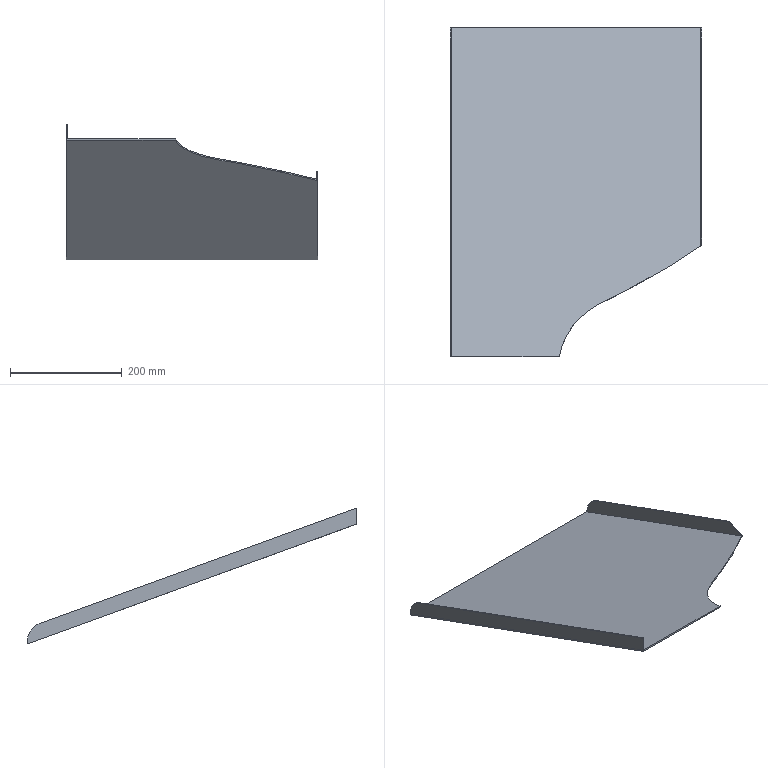Part | NX | features solid 2 | 1 solid | 15 faces | box 450 x 590 x 243.475 mm | volume 550261 mm3 | plane 11 | spline 2 | cylinder 2 | commonest cylinder face diameters 70 x2
STEP:
#1=CARTESIAN_POINT('',(-1002.,620.,-276.254));
#2=VERTEX_POINT('',#1);
#3=CARTESIAN_POINT('',(-1448.,620.,-276.254));
#4=VERTEX_POINT('',#3);
#5=CARTESIAN_POINT('',(-1000.,620.,-276.254));
#6=DIRECTION('',(-1.,0.,0.));
#7=VECTOR('',#6,1000.);
#8=LINE('',#5,#7);
#9=EDGE_CURVE('',#2,#4,#8,.T.);
#10=ORIENTED_EDGE('',*,*,#9,.T.);
#11=CARTESIAN_POINT('',(-1448.,30.,-61.511));
#12=VERTEX_POINT('',#11);
#13=CARTESIAN_POINT('',(-1448.,10.,-54.232));
#14=DIRECTION('',(0.,0.9397,-0.342));
#15=VECTOR('',#14,1000.);
#16=LINE('',#13,#15);
#17=EDGE_CURVE('',#12,#4,#16,.T.);
#18=ORIENTED_EDGE('',*,*,#17,.F.);
#19=CARTESIAN_POINT('',(-1254.916,30.,-61.511));
#20=VERTEX_POINT('',#19);
#21=CARTESIAN_POINT('',(-1445.,30.,-61.511));
#22=DIRECTION('',(1.,0.,0.));
#23=VECTOR('',#22,1000.);
#24=LINE('',#21,#23);
#25=EDGE_CURVE('',#20,#12,#24,.F.);
#26=ORIENTED_EDGE('',*,*,#25,.F.);
#27=CARTESIAN_POINT('',(-1059.954,190.696,-120.));
#28=VERTEX_POINT('',#27);
#29=CARTESIAN_POINT('',(-1059.954,190.696,-120.));
#30=CARTESIAN_POINT('',(-1064.698,187.84,-118.96));
#31=CARTESIAN_POINT('',(-1074.259,182.234,-116.92));
#32=CARTESIAN_POINT('',(-1088.653,173.903,-113.888));
#33=CARTESIAN_POINT('',(-1103.077,165.617,-110.872));
#34=CARTESIAN_POINT('',(-1122.557,154.937,-106.985));
#35=CARTESIAN_POINT('',(-1147.26,142.109,-102.316));
#36=CARTESIAN_POINT('',(-1172.64,130.297,-98.016));
#37=CARTESIAN_POINT('',(-1192.179,119.686,-94.154));
#38=CARTESIAN_POINT('',(-1205.944,110.685,-90.878));
#39=CARTESIAN_POINT('',(-1218.377,100.126,-87.035));
#40=CARTESIAN_POINT('',(-1229.411,87.869,-82.574));
#41=CARTESIAN_POINT('',(-1238.508,74.677,-77.773));
#42=CARTESIAN_POINT('',(-1244.626,62.872,-73.476));
#43=CARTESIAN_POINT('',(-1248.718,52.937,-69.86));
#44=CARTESIAN_POINT('',(-1252.053,42.833,-66.182));
#45=CARTESIAN_POINT('',(-1253.907,35.157,-63.388));
#46=CARTESIAN_POINT('',(-1254.916,30.,-61.511));
#47=B_SPLINE_CURVE_WITH_KNOTS('',3,(#29,#30,#31,#32,#33,#34,#35,#36,#37,#38,#39,#40,#41,#42,#43,#44,#45,#46),.UNSPECIFIED.,.F.,.F.,(4,1,1,1,1,1,1,1,1,1,1,1,1,1,1,4),(1.07,1.086,1.103,1.12,1.137,1.171,1.205,1.222,1.239,1.256,1.273,1.289,1.306,1.315,1.323,1.34),.UNSPECIFIED.);
#48=EDGE_CURVE('',#20,#28,#47,.F.);
#49=ORIENTED_EDGE('',*,*,#48,.T.);
#50=CARTESIAN_POINT('',(-1000.,229.424,-134.096));
#51=VERTEX_POINT('',#50);
#52=CARTESIAN_POINT('',(-1000.,229.424,-134.096));
#53=CARTESIAN_POINT('',(-1009.962,222.922,-131.729));
#54=CARTESIAN_POINT('',(-1029.91,209.956,-127.01));
#55=CARTESIAN_POINT('',(-1049.758,196.836,-122.235));
#56=CARTESIAN_POINT('',(-1059.954,190.696,-120.));
#57=B_SPLINE_CURVE_WITH_KNOTS('',3,(#52,#53,#54,#55,#56),.UNSPECIFIED.,.F.,.F.,(4,1,4),(0.3322,0.3686,0.405),.UNSPECIFIED.);
#58=EDGE_CURVE('',#51,#28,#57,.T.);
#59=ORIENTED_EDGE('',*,*,#58,.F.);
#60=CARTESIAN_POINT('',(-1002.,229.424,-134.096));
#61=VERTEX_POINT('',#60);
#62=CARTESIAN_POINT('',(-1000.,229.424,-134.096));
#63=DIRECTION('',(1.,0.,0.));
#64=VECTOR('',#63,1000.);
#65=LINE('',#62,#64);
#66=EDGE_CURVE('',#51,#61,#65,.F.);
#67=ORIENTED_EDGE('',*,*,#66,.T.);
#68=CARTESIAN_POINT('',(-1002.,229.424,-134.096));
#69=DIRECTION('',(0.,0.9397,-0.342));
#70=VECTOR('',#69,1000.);
#71=LINE('',#68,#70);
#72=EDGE_CURVE('',#61,#2,#71,.T.);
#73=ORIENTED_EDGE('',*,*,#72,.T.);
#74=EDGE_LOOP('',(#10,#18,#26,#49,#59,#67,#73));
#75=FACE_BOUND('',#74,.T.);
#76=CARTESIAN_POINT('',(-1000.,352.962,-179.06));
#77=DIRECTION('',(0.,-0.342,-0.9397));
#78=DIRECTION('',(0.,0.9397,-0.342));
#79=AXIS2_PLACEMENT_3D('',#76,#77,#78);
#80=PLANE('',#79);
#81=ADVANCED_FACE('',(#75),#80,.F.);
#82=CARTESIAN_POINT('',(-1069.813,184.849,-120.));
#83=VERTEX_POINT('',#82);
#84=CARTESIAN_POINT('',(-1000.,229.424,-136.224));
#85=VERTEX_POINT('',#84);
#86=CARTESIAN_POINT('',(-1069.813,184.849,-120.));
#87=CARTESIAN_POINT('',(-1063.841,188.35,-121.274));
#88=CARTESIAN_POINT('',(-1051.942,195.415,-123.846));
#89=CARTESIAN_POINT('',(-1028.916,210.612,-129.377));
#90=CARTESIAN_POINT('',(-1011.554,221.882,-133.479));
#91=CARTESIAN_POINT('',(-1000.,229.424,-136.224));
#92=B_SPLINE_CURVE_WITH_KNOTS('',3,(#86,#87,#88,#89,#90,#91),.UNSPECIFIED.,.F.,.F.,(4,1,1,4),(0.,0.0211,0.0422,0.0844),.UNSPECIFIED.);
#93=EDGE_CURVE('',#83,#85,#92,.T.);
#94=ORIENTED_EDGE('',*,*,#93,.F.);
#95=CARTESIAN_POINT('',(-1254.916,30.,-63.64));
#96=VERTEX_POINT('',#95);
#97=CARTESIAN_POINT('',(-1069.813,184.849,-120.));
#98=CARTESIAN_POINT('',(-1074.377,182.173,-119.026));
#99=CARTESIAN_POINT('',(-1083.541,176.877,-117.099));
#100=CARTESIAN_POINT('',(-1101.846,166.25,-113.231));
#101=CARTESIAN_POINT('',(-1125.083,153.491,-108.587));
#102=CARTESIAN_POINT('',(-1153.595,139.117,-103.355));
#103=CARTESIAN_POINT('',(-1177.787,127.749,-99.218));
#104=CARTESIAN_POINT('',(-1196.15,117.253,-95.397));
#105=CARTESIAN_POINT('',(-1209.224,108.178,-92.094));
#106=CARTESIAN_POINT('',(-1220.824,97.576,-88.235));
#107=CARTESIAN_POINT('',(-1230.91,85.914,-83.991));
#108=CARTESIAN_POINT('',(-1239.501,72.925,-79.263));
#109=CARTESIAN_POINT('',(-1246.413,59.227,-74.278));
#110=CARTESIAN_POINT('',(-1251.568,44.932,-69.074));
#111=CARTESIAN_POINT('',(-1253.944,34.97,-65.449));
#112=CARTESIAN_POINT('',(-1254.916,30.,-63.64));
#113=B_SPLINE_CURVE_WITH_KNOTS('',3,(#97,#98,#99,#100,#101,#102,#103,#104,#105,#106,#107,#108,#109,#110,#111,#112),.UNSPECIFIED.,.F.,.F.,(4,1,1,1,1,1,1,1,1,1,1,1,1,4),(1.112,1.128,1.144,1.177,1.209,1.241,1.257,1.274,1.29,1.306,1.322,1.338,1.354,1.371),.UNSPECIFIED.);
#114=EDGE_CURVE('',#83,#96,#113,.T.);
#115=ORIENTED_EDGE('',*,*,#114,.T.);
#116=CARTESIAN_POINT('',(-1450.,30.,-63.64));
#117=VERTEX_POINT('',#116);
#118=CARTESIAN_POINT('',(-1000.,30.,-63.64));
#119=DIRECTION('',(-1.,0.,0.));
#120=VECTOR('',#119,1000.);
#121=LINE('',#118,#120);
#122=EDGE_CURVE('',#96,#117,#121,.T.);
#123=ORIENTED_EDGE('',*,*,#122,.T.);
#124=CARTESIAN_POINT('',(-1450.,620.,-278.382));
#125=VERTEX_POINT('',#124);
#126=CARTESIAN_POINT('',(-1450.,352.278,-180.939));
#127=DIRECTION('',(0.,-0.9397,0.342));
#128=VECTOR('',#127,1000.);
#129=LINE('',#126,#128);
#130=EDGE_CURVE('',#117,#125,#129,.F.);
#131=ORIENTED_EDGE('',*,*,#130,.T.);
#132=CARTESIAN_POINT('',(-1000.,620.,-278.382));
#133=VERTEX_POINT('',#132);
#134=CARTESIAN_POINT('',(50.,620.,-278.382));
#135=DIRECTION('',(1.,0.,0.));
#136=VECTOR('',#135,1000.);
#137=LINE('',#134,#136);
#138=EDGE_CURVE('',#133,#125,#137,.F.);
#139=ORIENTED_EDGE('',*,*,#138,.F.);
#140=CARTESIAN_POINT('',(-1000.,352.278,-180.939));
#141=DIRECTION('',(0.,0.9397,-0.342));
#142=VECTOR('',#141,1000.);
#143=LINE('',#140,#142);
#144=EDGE_CURVE('',#85,#133,#143,.T.);
#145=ORIENTED_EDGE('',*,*,#144,.F.);
#146=EDGE_LOOP('',(#94,#115,#123,#131,#139,#145));
#147=FACE_BOUND('',#146,.T.);
#148=CARTESIAN_POINT('',(-1000.,352.278,-180.939));
#149=DIRECTION('',(0.,-0.342,-0.9397));
#150=DIRECTION('',(0.,0.9397,-0.342));
#151=AXIS2_PLACEMENT_3D('',#148,#149,#150);
#152=PLANE('',#151);
#153=ADVANCED_FACE('',(#147),#152,.T.);
#154=CARTESIAN_POINT('',(-1000.,261.467,-119.154));
#155=VERTEX_POINT('',#154);
#156=CARTESIAN_POINT('',(-1000.,596.971,-241.267));
#157=VERTEX_POINT('',#156);
#158=CARTESIAN_POINT('',(-1000.,237.975,-110.603));
#159=DIRECTION('',(0.,0.9397,-0.342));
#160=VECTOR('',#159,1000.);
#161=LINE('',#158,#160);
#162=EDGE_CURVE('',#155,#157,#161,.T.);
#163=ORIENTED_EDGE('',*,*,#162,.F.);
#164=CARTESIAN_POINT('',(-1000.,312.393,-95.407));
#165=DIRECTION('',(0.,0.9063,0.4226));
#166=VECTOR('',#165,1000.);
#167=LINE('',#164,#166);
#168=EDGE_CURVE('',#155,#51,#167,.F.);
#169=ORIENTED_EDGE('',*,*,#168,.T.);
#170=CARTESIAN_POINT('',(-1000.,229.424,-132.987));
#171=DIRECTION('',(0.,0.,-1.));
#172=VECTOR('',#171,1000.);
#173=LINE('',#170,#172);
#174=EDGE_CURVE('',#51,#85,#173,.T.);
#175=ORIENTED_EDGE('',*,*,#174,.T.);
#176=ORIENTED_EDGE('',*,*,#144,.T.);
#177=CARTESIAN_POINT('',(-1000.,620.,-274.157));
#178=VERTEX_POINT('',#177);
#179=CARTESIAN_POINT('',(-1000.,620.,-570.));
#180=DIRECTION('',(0.,0.,1.));
#181=VECTOR('',#180,1000.);
#182=LINE('',#179,#181);
#183=EDGE_CURVE('',#133,#178,#182,.T.);
#184=ORIENTED_EDGE('',*,*,#183,.T.);
#185=CARTESIAN_POINT('',(-1000.,585.,-274.157));
#186=DIRECTION('',(1.,0.,0.));
#187=DIRECTION('',(0.,0.,-1.));
#188=AXIS2_PLACEMENT_3D('',#185,#186,#187);
#189=CIRCLE('',#188,35.);
#190=EDGE_CURVE('',#178,#157,#189,.T.);
#191=ORIENTED_EDGE('',*,*,#190,.T.);
#192=EDGE_LOOP('',(#163,#169,#175,#176,#184,#191));
#193=FACE_BOUND('',#192,.T.);
#194=CARTESIAN_POINT('',(-1000.,352.278,-180.939));
#195=DIRECTION('',(1.,0.,0.));
#196=DIRECTION('',(0.,0.,-1.));
#197=AXIS2_PLACEMENT_3D('',#194,#195,#196);
#198=PLANE('',#197);
#199=ADVANCED_FACE('',(#193),#198,.T.);
#200=CARTESIAN_POINT('',(-1450.,620.,-274.157));
#201=VERTEX_POINT('',#200);
#202=CARTESIAN_POINT('',(-1450.,620.,-570.));
#203=DIRECTION('',(0.,0.,1.));
#204=VECTOR('',#203,1000.);
#205=LINE('',#202,#204);
#206=EDGE_CURVE('',#125,#201,#205,.T.);
#207=ORIENTED_EDGE('',*,*,#206,.T.);
#208=CARTESIAN_POINT('',(-1448.,620.,-274.157));
#209=VERTEX_POINT('',#208);
#210=CARTESIAN_POINT('',(-1468.,620.,-274.157));
#211=DIRECTION('',(-1.,0.,0.));
#212=VECTOR('',#211,1000.);
#213=LINE('',#210,#212);
#214=EDGE_CURVE('',#201,#209,#213,.F.);
#215=ORIENTED_EDGE('',*,*,#214,.T.);
#216=CARTESIAN_POINT('',(-1448.,620.,-570.));
#217=DIRECTION('',(0.,0.,1.));
#218=VECTOR('',#217,1000.);
#219=LINE('',#216,#218);
#220=EDGE_CURVE('',#4,#209,#219,.T.);
#221=ORIENTED_EDGE('',*,*,#220,.F.);
#222=ORIENTED_EDGE('',*,*,#9,.F.);
#223=CARTESIAN_POINT('',(-1002.,620.,-274.157));
#224=VERTEX_POINT('',#223);
#225=CARTESIAN_POINT('',(-1002.,620.,-570.));
#226=DIRECTION('',(0.,0.,1.));
#227=VECTOR('',#226,1000.);
#228=LINE('',#225,#227);
#229=EDGE_CURVE('',#2,#224,#228,.T.);
#230=ORIENTED_EDGE('',*,*,#229,.T.);
#231=CARTESIAN_POINT('',(50.,620.,-274.157));
#232=DIRECTION('',(-1.,0.,0.));
#233=VECTOR('',#232,1000.);
#234=LINE('',#231,#233);
#235=EDGE_CURVE('',#224,#178,#234,.F.);
#236=ORIENTED_EDGE('',*,*,#235,.T.);
#237=ORIENTED_EDGE('',*,*,#183,.F.);
#238=ORIENTED_EDGE('',*,*,#138,.T.);
#239=EDGE_LOOP('',(#207,#215,#221,#222,#230,#236,#237,#238));
#240=FACE_BOUND('',#239,.T.);
#241=CARTESIAN_POINT('',(50.,620.,-570.));
#242=DIRECTION('',(0.,-1.,0.));
#243=DIRECTION('',(-1.,0.,0.));
#244=AXIS2_PLACEMENT_3D('',#241,#242,#243);
#245=PLANE('',#244);
#246=ADVANCED_FACE('',(#240),#245,.F.);
#247=CARTESIAN_POINT('',(-1450.,30.,-34.907));
#248=VERTEX_POINT('',#247);
#249=CARTESIAN_POINT('',(-1448.,30.,-34.907));
#250=VERTEX_POINT('',#249);
#251=CARTESIAN_POINT('',(-1445.,30.,-34.907));
#252=DIRECTION('',(1.,0.,0.));
#253=VECTOR('',#252,1000.);
#254=LINE('',#251,#253);
#255=EDGE_CURVE('',#248,#250,#254,.T.);
#256=ORIENTED_EDGE('',*,*,#255,.F.);
#257=CARTESIAN_POINT('',(-1450.,30.,0.));
#258=DIRECTION('',(0.,0.,-1.));
#259=VECTOR('',#258,1000.);
#260=LINE('',#257,#259);
#261=EDGE_CURVE('',#117,#248,#260,.F.);
#262=ORIENTED_EDGE('',*,*,#261,.F.);
#263=ORIENTED_EDGE('',*,*,#122,.F.);
#264=CARTESIAN_POINT('',(-1254.916,30.,-69.855));
#265=DIRECTION('',(0.,0.,-1.));
#266=VECTOR('',#265,1000.);
#267=LINE('',#264,#266);
#268=EDGE_CURVE('',#96,#20,#267,.F.);
#269=ORIENTED_EDGE('',*,*,#268,.T.);
#270=ORIENTED_EDGE('',*,*,#25,.T.);
#271=CARTESIAN_POINT('',(-1448.,30.,-54.232));
#272=DIRECTION('',(0.,0.,-1.));
#273=VECTOR('',#272,1000.);
#274=LINE('',#271,#273);
#275=EDGE_CURVE('',#12,#250,#274,.F.);
#276=ORIENTED_EDGE('',*,*,#275,.T.);
#277=EDGE_LOOP('',(#256,#262,#263,#269,#270,#276));
#278=FACE_BOUND('',#277,.T.);
#279=CARTESIAN_POINT('',(-1445.,30.,-180.));
#280=DIRECTION('',(0.,-1.,0.));
#281=DIRECTION('',(1.,0.,0.));
#282=AXIS2_PLACEMENT_3D('',#279,#280,#281);
#283=PLANE('',#282);
#284=ADVANCED_FACE('',(#278),#283,.T.);
#285=ORIENTED_EDGE('',*,*,#261,.T.);
#286=CARTESIAN_POINT('',(-1450.,596.971,-241.267));
#287=VERTEX_POINT('',#286);
#288=CARTESIAN_POINT('',(-1450.,18.551,-30.74));
#289=DIRECTION('',(0.,-0.9397,0.342));
#290=VECTOR('',#289,1000.);
#291=LINE('',#288,#290);
#292=EDGE_CURVE('',#248,#287,#291,.F.);
#293=ORIENTED_EDGE('',*,*,#292,.T.);
#294=CARTESIAN_POINT('',(-1450.,585.,-274.157));
#295=DIRECTION('',(1.,0.,0.));
#296=DIRECTION('',(0.,0.,-1.));
#297=AXIS2_PLACEMENT_3D('',#294,#295,#296);
#298=CIRCLE('',#297,35.);
#299=EDGE_CURVE('',#287,#201,#298,.F.);
#300=ORIENTED_EDGE('',*,*,#299,.T.);
#301=ORIENTED_EDGE('',*,*,#206,.F.);
#302=ORIENTED_EDGE('',*,*,#130,.F.);
#303=EDGE_LOOP('',(#285,#293,#300,#301,#302));
#304=FACE_BOUND('',#303,.T.);
#305=CARTESIAN_POINT('',(-1450.,580.,0.));
#306=DIRECTION('',(1.,0.,0.));
#307=DIRECTION('',(0.,0.,-1.));
#308=AXIS2_PLACEMENT_3D('',#305,#306,#307);
#309=PLANE('',#308);
#310=ADVANCED_FACE('',(#304),#309,.F.);
#311=CARTESIAN_POINT('',(-1059.954,190.696,-120.));
#312=CARTESIAN_POINT('',(-1063.22,188.73,-120.));
#313=CARTESIAN_POINT('',(-1066.511,186.784,-120.));
#314=CARTESIAN_POINT('',(-1069.813,184.849,-120.));
#315=B_SPLINE_CURVE_WITH_KNOTS('',3,(#311,#312,#313,#314),.UNSPECIFIED.,.F.,.F.,(4,4),(0.004472,0.007483),.UNSPECIFIED.);
#316=EDGE_CURVE('',#83,#28,#315,.F.);
#317=ORIENTED_EDGE('',*,*,#316,.T.);
#318=ORIENTED_EDGE('',*,*,#48,.F.);
#319=ORIENTED_EDGE('',*,*,#268,.F.);
#320=ORIENTED_EDGE('',*,*,#114,.F.);
#321=EDGE_LOOP('',(#317,#318,#319,#320));
#322=FACE_BOUND('',#321,.T.);
#323=CARTESIAN_POINT('',(-1058.635,191.493,-61.16));
#324=CARTESIAN_POINT('',(-1058.635,191.493,-120.));
#325=CARTESIAN_POINT('',(-1067.844,185.918,-61.16));
#326=CARTESIAN_POINT('',(-1067.844,185.918,-120.));
#327=CARTESIAN_POINT('',(-1081.973,177.783,-61.16));
#328=CARTESIAN_POINT('',(-1081.973,177.783,-120.));
#329=CARTESIAN_POINT('',(-1100.678,166.961,-61.16));
#330=CARTESIAN_POINT('',(-1100.678,166.961,-120.));
#331=CARTESIAN_POINT('',(-1119.607,156.53,-61.16));
#332=CARTESIAN_POINT('',(-1119.607,156.53,-120.));
#333=CARTESIAN_POINT('',(-1143.47,143.982,-61.16));
#334=CARTESIAN_POINT('',(-1143.47,143.982,-120.));
#335=CARTESIAN_POINT('',(-1167.958,132.51,-61.16));
#336=CARTESIAN_POINT('',(-1167.958,132.51,-120.));
#337=CARTESIAN_POINT('',(-1187.526,122.355,-61.16));
#338=CARTESIAN_POINT('',(-1187.526,122.355,-120.));
#339=CARTESIAN_POINT('',(-1201.808,113.614,-61.16));
#340=CARTESIAN_POINT('',(-1201.808,113.614,-120.));
#341=CARTESIAN_POINT('',(-1213.002,104.922,-61.16));
#342=CARTESIAN_POINT('',(-1213.002,104.922,-120.));
#343=CARTESIAN_POINT('',(-1221.094,96.979,-61.16));
#344=CARTESIAN_POINT('',(-1221.094,96.979,-120.));
#345=CARTESIAN_POINT('',(-1228.627,88.632,-61.16));
#346=CARTESIAN_POINT('',(-1228.627,88.632,-120.));
#347=CARTESIAN_POINT('',(-1237.052,77.161,-61.16));
#348=CARTESIAN_POINT('',(-1237.052,77.161,-120.));
#349=CARTESIAN_POINT('',(-1243.739,64.75,-61.16));
#350=CARTESIAN_POINT('',(-1243.739,64.75,-120.));
#351=CARTESIAN_POINT('',(-1248.189,54.365,-61.16));
#352=CARTESIAN_POINT('',(-1248.189,54.365,-120.));
#353=CARTESIAN_POINT('',(-1251.865,43.619,-61.16));
#354=CARTESIAN_POINT('',(-1251.865,43.619,-120.));
#355=CARTESIAN_POINT('',(-1253.841,35.493,-61.16));
#356=CARTESIAN_POINT('',(-1253.841,35.493,-120.));
#357=CARTESIAN_POINT('',(-1254.916,30.,-61.16));
#358=CARTESIAN_POINT('',(-1254.916,30.,-120.));
#359=B_SPLINE_SURFACE_WITH_KNOTS('',3,1,((#323,#324),(#325,#326),(#327,#328),(#329,#330),(#331,#332),(#333,#334),(#335,#336),(#337,#338),(#339,#340),(#341,#342),(#343,#344),(#345,#346),(#347,#348),(#349,#350),(#351,#352),(#353,#354),(#355,#356),(#357,#358)),.SURF_OF_LINEAR_EXTRUSION.,.F.,.F.,.F.,(4,1,1,1,1,1,1,1,1,1,1,1,1,1,1,4),(2,2),(0.004067,0.01257,0.01683,0.02108,0.02959,0.03809,0.04234,0.0466,0.05085,0.05298,0.0551,0.05936,0.06361,0.06574,0.06786,0.07212),(0.,1.),.UNSPECIFIED.);
#360=ADVANCED_FACE('',(#322),#359,.T.);
#361=ORIENTED_EDGE('',*,*,#93,.T.);
#362=ORIENTED_EDGE('',*,*,#174,.F.);
#363=ORIENTED_EDGE('',*,*,#58,.T.);
#364=ORIENTED_EDGE('',*,*,#316,.F.);
#365=EDGE_LOOP('',(#361,#362,#363,#364));
#366=FACE_BOUND('',#365,.T.);
#367=CARTESIAN_POINT('',(-1000.,229.424,-120.));
#368=CARTESIAN_POINT('',(-1000.,229.424,-136.321));
#369=CARTESIAN_POINT('',(-1005.833,225.617,-120.));
#370=CARTESIAN_POINT('',(-1005.833,225.617,-136.321));
#371=CARTESIAN_POINT('',(-1017.502,217.997,-120.));
#372=CARTESIAN_POINT('',(-1017.502,217.997,-136.321));
#373=CARTESIAN_POINT('',(-1032.069,208.499,-120.));
#374=CARTESIAN_POINT('',(-1032.069,208.499,-136.321));
#375=CARTESIAN_POINT('',(-1043.763,200.845,-120.));
#376=CARTESIAN_POINT('',(-1043.763,200.845,-136.321));
#377=CARTESIAN_POINT('',(-1055.309,193.391,-120.));
#378=CARTESIAN_POINT('',(-1055.309,193.391,-136.321));
#379=CARTESIAN_POINT('',(-1064.251,188.106,-120.));
#380=CARTESIAN_POINT('',(-1064.251,188.106,-136.321));
#381=CARTESIAN_POINT('',(-1070.242,184.597,-120.));
#382=CARTESIAN_POINT('',(-1070.242,184.597,-136.321));
#383=B_SPLINE_SURFACE_WITH_KNOTS('',3,1,((#367,#368),(#369,#370),(#371,#372),(#373,#374),(#375,#376),(#377,#378),(#379,#380),(#381,#382)),.SURF_OF_LINEAR_EXTRUSION.,.F.,.F.,.F.,(4,1,1,1,1,4),(2,2),(-0.01423,-0.008766,-0.003306,-0.0005765,0.002153,0.007613),(0.,1.),.UNSPECIFIED.);
#384=ADVANCED_FACE('',(#366),#383,.T.);
#385=CARTESIAN_POINT('',(-1002.,261.467,-119.154));
#386=VERTEX_POINT('',#385);
#387=CARTESIAN_POINT('',(-1002.,596.971,-241.267));
#388=VERTEX_POINT('',#387);
#389=CARTESIAN_POINT('',(-1002.,237.975,-110.603));
#390=DIRECTION('',(0.,0.9397,-0.342));
#391=VECTOR('',#390,1000.);
#392=LINE('',#389,#391);
#393=EDGE_CURVE('',#386,#388,#392,.T.);
#394=ORIENTED_EDGE('',*,*,#393,.F.);
#395=CARTESIAN_POINT('',(-1000.,261.467,-119.154));
#396=DIRECTION('',(1.,0.,0.));
#397=VECTOR('',#396,1000.);
#398=LINE('',#395,#397);
#399=EDGE_CURVE('',#386,#155,#398,.T.);
#400=ORIENTED_EDGE('',*,*,#399,.T.);
#401=ORIENTED_EDGE('',*,*,#162,.T.);
#402=CARTESIAN_POINT('',(-1000.,596.971,-241.267));
#403=DIRECTION('',(-1.,0.,0.));
#404=VECTOR('',#403,1000.);
#405=LINE('',#402,#404);
#406=EDGE_CURVE('',#157,#388,#405,.T.);
#407=ORIENTED_EDGE('',*,*,#406,.T.);
#408=EDGE_LOOP('',(#394,#400,#401,#407));
#409=FACE_BOUND('',#408,.T.);
#410=CARTESIAN_POINT('',(-1000.,237.975,-110.603));
#411=DIRECTION('',(0.,-0.342,-0.9397));
#412=DIRECTION('',(0.,0.9397,-0.342));
#413=AXIS2_PLACEMENT_3D('',#410,#411,#412);
#414=PLANE('',#413);
#415=ADVANCED_FACE('',(#409),#414,.F.);
#416=ORIENTED_EDGE('',*,*,#72,.F.);
#417=CARTESIAN_POINT('',(-1002.,229.424,-134.096));
#418=DIRECTION('',(0.,-0.9063,-0.4226));
#419=VECTOR('',#418,1000.);
#420=LINE('',#417,#419);
#421=EDGE_CURVE('',#61,#386,#420,.F.);
#422=ORIENTED_EDGE('',*,*,#421,.T.);
#423=ORIENTED_EDGE('',*,*,#393,.T.);
#424=CARTESIAN_POINT('',(-1002.,585.,-274.157));
#425=DIRECTION('',(1.,0.,0.));
#426=DIRECTION('',(0.,0.,-1.));
#427=AXIS2_PLACEMENT_3D('',#424,#425,#426);
#428=CIRCLE('',#427,35.);
#429=EDGE_CURVE('',#388,#224,#428,.F.);
#430=ORIENTED_EDGE('',*,*,#429,.T.);
#431=ORIENTED_EDGE('',*,*,#229,.F.);
#432=EDGE_LOOP('',(#416,#422,#423,#430,#431));
#433=FACE_BOUND('',#432,.T.);
#434=CARTESIAN_POINT('',(-1002.,229.424,-134.096));
#435=DIRECTION('',(1.,0.,0.));
#436=DIRECTION('',(0.,0.,-1.));
#437=AXIS2_PLACEMENT_3D('',#434,#435,#436);
#438=PLANE('',#437);
#439=ADVANCED_FACE('',(#433),#438,.F.);
#440=ORIENTED_EDGE('',*,*,#292,.F.);
#441=ORIENTED_EDGE('',*,*,#255,.T.);
#442=CARTESIAN_POINT('',(-1448.,596.971,-241.267));
#443=VERTEX_POINT('',#442);
#444=CARTESIAN_POINT('',(-1448.,18.551,-30.74));
#445=DIRECTION('',(0.,-0.9397,0.342));
#446=VECTOR('',#445,1000.);
#447=LINE('',#444,#446);
#448=EDGE_CURVE('',#250,#443,#447,.F.);
#449=ORIENTED_EDGE('',*,*,#448,.T.);
#450=CARTESIAN_POINT('',(-1470.,596.971,-241.267));
#451=DIRECTION('',(1.,0.,0.));
#452=VECTOR('',#451,1000.);
#453=LINE('',#450,#452);
#454=EDGE_CURVE('',#443,#287,#453,.F.);
#455=ORIENTED_EDGE('',*,*,#454,.T.);
#456=EDGE_LOOP('',(#440,#441,#449,#455));
#457=FACE_BOUND('',#456,.T.);
#458=CARTESIAN_POINT('',(-1470.,18.551,-30.74));
#459=DIRECTION('',(0.,-0.342,-0.9397));
#460=DIRECTION('',(0.,0.9397,-0.342));
#461=AXIS2_PLACEMENT_3D('',#458,#459,#460);
#462=PLANE('',#461);
#463=ADVANCED_FACE('',(#457),#462,.F.);
#464=ORIENTED_EDGE('',*,*,#448,.F.);
#465=ORIENTED_EDGE('',*,*,#275,.F.);
#466=ORIENTED_EDGE('',*,*,#17,.T.);
#467=ORIENTED_EDGE('',*,*,#220,.T.);
#468=CARTESIAN_POINT('',(-1448.,585.,-274.157));
#469=DIRECTION('',(1.,0.,0.));
#470=DIRECTION('',(0.,0.,-1.));
#471=AXIS2_PLACEMENT_3D('',#468,#469,#470);
#472=CIRCLE('',#471,35.);
#473=EDGE_CURVE('',#209,#443,#472,.T.);
#474=ORIENTED_EDGE('',*,*,#473,.T.);
#475=EDGE_LOOP('',(#464,#465,#466,#467,#474));
#476=FACE_BOUND('',#475,.T.);
#477=CARTESIAN_POINT('',(-1448.,10.,-54.232));
#478=DIRECTION('',(1.,0.,0.));
#479=DIRECTION('',(0.,0.,-1.));
#480=AXIS2_PLACEMENT_3D('',#477,#478,#479);
#481=PLANE('',#480);
#482=ADVANCED_FACE('',(#476),#481,.T.);
#483=ORIENTED_EDGE('',*,*,#190,.F.);
#484=ORIENTED_EDGE('',*,*,#235,.F.);
#485=ORIENTED_EDGE('',*,*,#429,.F.);
#486=ORIENTED_EDGE('',*,*,#406,.F.);
#487=EDGE_LOOP('',(#483,#484,#485,#486));
#488=FACE_BOUND('',#487,.T.);
#489=CARTESIAN_POINT('',(-1000.,585.,-274.157));
#490=DIRECTION('',(-1.,0.,0.));
#491=DIRECTION('',(0.,0.,1.));
#492=AXIS2_PLACEMENT_3D('',#489,#490,#491);
#493=CYLINDRICAL_SURFACE('',#492,35.);
#494=ADVANCED_FACE('',(#488),#493,.T.);
#495=ORIENTED_EDGE('',*,*,#299,.F.);
#496=ORIENTED_EDGE('',*,*,#454,.F.);
#497=ORIENTED_EDGE('',*,*,#473,.F.);
#498=ORIENTED_EDGE('',*,*,#214,.F.);
#499=EDGE_LOOP('',(#495,#496,#497,#498));
#500=FACE_BOUND('',#499,.T.);
#501=CARTESIAN_POINT('',(50.,585.,-274.157));
#502=DIRECTION('',(1.,0.,0.));
#503=DIRECTION('',(0.,0.,-1.));
#504=AXIS2_PLACEMENT_3D('',#501,#502,#503);
#505=CYLINDRICAL_SURFACE('',#504,35.);
#506=ADVANCED_FACE('',(#500),#505,.T.);
#507=ORIENTED_EDGE('',*,*,#168,.F.);
#508=ORIENTED_EDGE('',*,*,#399,.F.);
#509=ORIENTED_EDGE('',*,*,#421,.F.);
#510=ORIENTED_EDGE('',*,*,#66,.F.);
#511=EDGE_LOOP('',(#507,#508,#509,#510));
#512=FACE_BOUND('',#511,.T.);
#513=CARTESIAN_POINT('',(-1000.,229.424,-134.096));
#514=DIRECTION('',(0.,0.4226,-0.9063));
#515=DIRECTION('',(0.,0.9063,0.4226));
#516=AXIS2_PLACEMENT_3D('',#513,#514,#515);
#517=PLANE('',#516);
#518=ADVANCED_FACE('',(#512),#517,.F.);
#519=CLOSED_SHELL('',(#81,#153,#199,#246,#284,#310,#360,#384,#415,#439,#463,#482,#494,#506,#518));
#520=MANIFOLD_SOLID_BREP('',#519);
#521=(LENGTH_UNIT()NAMED_UNIT(*)SI_UNIT(.MILLI.,.METRE.));
#522=UNCERTAINTY_MEASURE_WITH_UNIT(LENGTH_MEASURE(0.0508),#521,'','');
#523=(NAMED_UNIT(*)PLANE_ANGLE_UNIT()SI_UNIT($,.RADIAN.));
#524=(NAMED_UNIT(*)SI_UNIT($,.STERADIAN.)SOLID_ANGLE_UNIT());
#525=(GEOMETRIC_REPRESENTATION_CONTEXT(3)GLOBAL_UNCERTAINTY_ASSIGNED_CONTEXT((#522))GLOBAL_UNIT_ASSIGNED_CONTEXT((#521,#523,#524))REPRESENTATION_CONTEXT('',''));
#526=ADVANCED_BREP_SHAPE_REPRESENTATION('',(#520),#525);